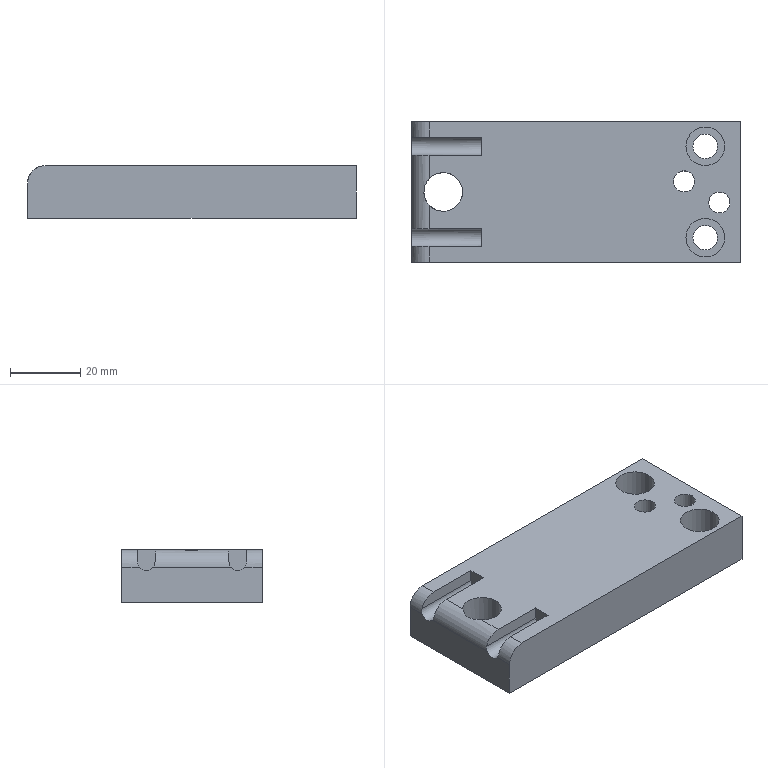Part | NX | features solid 2 | 1 solid | 26 faces | box 93.5 x 40 x 15 mm | volume 50400 mm3 | plane 14 | cylinder 12 | commonest cylinder face diameters 10 x3 11 x3 5 x2 6.001 x2 7 x2
STEP:
#1=CARTESIAN_POINT('',(481.,-15.5,-5.));
#2=VERTEX_POINT('',#1);
#3=CARTESIAN_POINT('',(481.,-10.5,-5.));
#4=VERTEX_POINT('',#3);
#5=CARTESIAN_POINT('',(481.,-13.,-5.));
#6=DIRECTION('',(1.,0.,0.));
#7=DIRECTION('',(0.,0.,1.));
#8=AXIS2_PLACEMENT_3D('',#5,#6,#7);
#9=CIRCLE('',#8,2.5);
#10=EDGE_CURVE('',#2,#4,#9,.T.);
#11=ORIENTED_EDGE('',*,*,#10,.F.);
#12=CARTESIAN_POINT('',(481.,-15.5,-1.5));
#13=VERTEX_POINT('',#12);
#14=CARTESIAN_POINT('',(481.,-15.5,25.));
#15=DIRECTION('',(0.,0.,-1.));
#16=VECTOR('',#15,1000.);
#17=LINE('',#14,#16);
#18=EDGE_CURVE('',#2,#13,#17,.F.);
#19=ORIENTED_EDGE('',*,*,#18,.T.);
#20=CARTESIAN_POINT('',(481.,-10.5,-1.5));
#21=VERTEX_POINT('',#20);
#22=CARTESIAN_POINT('',(481.,0.,-1.5));
#23=DIRECTION('',(0.,-1.,0.));
#24=VECTOR('',#23,1000.);
#25=LINE('',#22,#24);
#26=EDGE_CURVE('',#21,#13,#25,.T.);
#27=ORIENTED_EDGE('',*,*,#26,.F.);
#28=CARTESIAN_POINT('',(481.,-10.5,25.));
#29=DIRECTION('',(0.,0.,-1.));
#30=VECTOR('',#29,1000.);
#31=LINE('',#28,#30);
#32=EDGE_CURVE('',#4,#21,#31,.F.);
#33=ORIENTED_EDGE('',*,*,#32,.F.);
#34=EDGE_LOOP('',(#11,#19,#27,#33));
#35=FACE_BOUND('',#34,.T.);
#36=CARTESIAN_POINT('',(481.,-13.,-5.));
#37=DIRECTION('',(-1.,0.,0.));
#38=DIRECTION('',(0.,0.,1.));
#39=AXIS2_PLACEMENT_3D('',#36,#37,#38);
#40=PLANE('',#39);
#41=ADVANCED_FACE('',(#35),#40,.T.);
#42=CARTESIAN_POINT('',(461.,-11.,-6.5));
#43=VERTEX_POINT('',#42);
#44=CARTESIAN_POINT('',(461.23,-10.5,-5.));
#45=VERTEX_POINT('',#44);
#46=CARTESIAN_POINT('',(461.,-11.,-6.5));
#47=CARTESIAN_POINT('',(461.,-10.671,-6.061));
#48=CARTESIAN_POINT('',(461.066,-10.5,-5.521));
#49=CARTESIAN_POINT('',(461.23,-10.5,-5.));
#50=B_SPLINE_CURVE_WITH_KNOTS('',3,(#46,#47,#48,#49),.UNSPECIFIED.,.F.,.F.,(4,4),(0.,0.001624),.UNSPECIFIED.);
#51=EDGE_CURVE('',#43,#45,#50,.T.);
#52=ORIENTED_EDGE('',*,*,#51,.F.);
#53=CARTESIAN_POINT('',(461.,-15.,-6.5));
#54=VERTEX_POINT('',#53);
#55=CARTESIAN_POINT('',(461.,-13.,-5.));
#56=DIRECTION('',(-1.,0.,0.));
#57=DIRECTION('',(0.,0.,1.));
#58=AXIS2_PLACEMENT_3D('',#55,#56,#57);
#59=CIRCLE('',#58,2.5);
#60=EDGE_CURVE('',#54,#43,#59,.F.);
#61=ORIENTED_EDGE('',*,*,#60,.F.);
#62=CARTESIAN_POINT('',(461.23,-15.5,-5.));
#63=VERTEX_POINT('',#62);
#64=CARTESIAN_POINT('',(461.23,-15.5,-5.));
#65=CARTESIAN_POINT('',(461.068,-15.5,-5.516));
#66=CARTESIAN_POINT('',(461.,-15.329,-6.061));
#67=CARTESIAN_POINT('',(461.,-15.,-6.5));
#68=B_SPLINE_CURVE_WITH_KNOTS('',3,(#64,#65,#66,#67),.UNSPECIFIED.,.F.,.F.,(4,4),(0.01027,0.01189),.UNSPECIFIED.);
#69=EDGE_CURVE('',#63,#54,#68,.T.);
#70=ORIENTED_EDGE('',*,*,#69,.F.);
#71=CARTESIAN_POINT('',(451.,-15.5,-5.));
#72=DIRECTION('',(1.,0.,0.));
#73=VECTOR('',#72,1000.);
#74=LINE('',#71,#73);
#75=EDGE_CURVE('',#2,#63,#74,.F.);
#76=ORIENTED_EDGE('',*,*,#75,.F.);
#77=ORIENTED_EDGE('',*,*,#10,.T.);
#78=CARTESIAN_POINT('',(451.,-10.5,-5.));
#79=DIRECTION('',(1.,0.,0.));
#80=VECTOR('',#79,1000.);
#81=LINE('',#78,#80);
#82=EDGE_CURVE('',#45,#4,#81,.T.);
#83=ORIENTED_EDGE('',*,*,#82,.F.);
#84=EDGE_LOOP('',(#52,#61,#70,#76,#77,#83));
#85=FACE_BOUND('',#84,.T.);
#86=CARTESIAN_POINT('',(427.633,-13.,-5.));
#87=DIRECTION('',(1.,0.,0.));
#88=DIRECTION('',(0.,0.,-1.));
#89=AXIS2_PLACEMENT_3D('',#86,#87,#88);
#90=CYLINDRICAL_SURFACE('',#89,2.5);
#91=ADVANCED_FACE('',(#85),#90,.F.);
#92=CARTESIAN_POINT('',(466.,-10.5,-1.5));
#93=VERTEX_POINT('',#92);
#94=CARTESIAN_POINT('',(466.,-10.5,-6.5));
#95=DIRECTION('',(0.,1.,0.));
#96=DIRECTION('',(0.,0.,1.));
#97=AXIS2_PLACEMENT_3D('',#94,#95,#96);
#98=CIRCLE('',#97,5.);
#99=EDGE_CURVE('',#93,#45,#98,.F.);
#100=ORIENTED_EDGE('',*,*,#99,.T.);
#101=ORIENTED_EDGE('',*,*,#82,.T.);
#102=ORIENTED_EDGE('',*,*,#32,.T.);
#103=CARTESIAN_POINT('',(365.,-10.5,-1.5));
#104=DIRECTION('',(-1.,0.,0.));
#105=VECTOR('',#104,1000.);
#106=LINE('',#103,#105);
#107=EDGE_CURVE('',#21,#93,#106,.T.);
#108=ORIENTED_EDGE('',*,*,#107,.T.);
#109=EDGE_LOOP('',(#100,#101,#102,#108));
#110=FACE_BOUND('',#109,.T.);
#111=CARTESIAN_POINT('',(451.,-10.5,25.));
#112=DIRECTION('',(0.,1.,0.));
#113=DIRECTION('',(0.,0.,-1.));
#114=AXIS2_PLACEMENT_3D('',#111,#112,#113);
#115=PLANE('',#114);
#116=ADVANCED_FACE('',(#110),#115,.F.);
#117=CARTESIAN_POINT('',(466.,-15.5,-1.5));
#118=VERTEX_POINT('',#117);
#119=CARTESIAN_POINT('',(466.,-15.5,-6.5));
#120=DIRECTION('',(0.,-1.,0.));
#121=DIRECTION('',(0.,0.,-1.));
#122=AXIS2_PLACEMENT_3D('',#119,#120,#121);
#123=CIRCLE('',#122,5.);
#124=EDGE_CURVE('',#63,#118,#123,.F.);
#125=ORIENTED_EDGE('',*,*,#124,.T.);
#126=CARTESIAN_POINT('',(365.,-15.5,-1.5));
#127=DIRECTION('',(1.,0.,0.));
#128=VECTOR('',#127,1000.);
#129=LINE('',#126,#128);
#130=EDGE_CURVE('',#118,#13,#129,.T.);
#131=ORIENTED_EDGE('',*,*,#130,.T.);
#132=ORIENTED_EDGE('',*,*,#18,.F.);
#133=ORIENTED_EDGE('',*,*,#75,.T.);
#134=EDGE_LOOP('',(#125,#131,#132,#133));
#135=FACE_BOUND('',#134,.T.);
#136=CARTESIAN_POINT('',(451.,-15.5,25.));
#137=DIRECTION('',(0.,-1.,0.));
#138=DIRECTION('',(0.,0.,1.));
#139=AXIS2_PLACEMENT_3D('',#136,#137,#138);
#140=PLANE('',#139);
#141=ADVANCED_FACE('',(#135),#140,.F.);
#142=CARTESIAN_POINT('',(461.,11.,-6.5));
#143=VERTEX_POINT('',#142);
#144=CARTESIAN_POINT('',(461.,-29.,-6.5));
#145=DIRECTION('',(0.,-1.,0.));
#146=VECTOR('',#145,1000.);
#147=LINE('',#144,#146);
#148=EDGE_CURVE('',#43,#143,#147,.F.);
#149=ORIENTED_EDGE('',*,*,#148,.F.);
#150=ORIENTED_EDGE('',*,*,#51,.T.);
#151=ORIENTED_EDGE('',*,*,#99,.F.);
#152=CARTESIAN_POINT('',(466.,-3.775,-1.5));
#153=VERTEX_POINT('',#152);
#154=CARTESIAN_POINT('',(466.,0.,-1.5));
#155=DIRECTION('',(0.,-1.,0.));
#156=VECTOR('',#155,1000.);
#157=LINE('',#154,#156);
#158=EDGE_CURVE('',#153,#93,#157,.T.);
#159=ORIENTED_EDGE('',*,*,#158,.F.);
#160=CARTESIAN_POINT('',(466.,3.775,-1.5));
#161=VERTEX_POINT('',#160);
#162=CARTESIAN_POINT('',(466.,3.775,-1.5));
#163=CARTESIAN_POINT('',(465.037,2.755,-1.5));
#164=CARTESIAN_POINT('',(463.963,0.004291,-1.961));
#165=CARTESIAN_POINT('',(465.038,-2.755,-1.5));
#166=CARTESIAN_POINT('',(466.,-3.775,-1.5));
#167=B_SPLINE_CURVE_WITH_KNOTS('',3,(#162,#163,#164,#165,#166),.UNSPECIFIED.,.F.,.F.,(4,1,4),(0.,0.004144,0.008289),.UNSPECIFIED.);
#168=EDGE_CURVE('',#161,#153,#167,.T.);
#169=ORIENTED_EDGE('',*,*,#168,.F.);
#170=CARTESIAN_POINT('',(466.,10.5,-1.5));
#171=VERTEX_POINT('',#170);
#172=CARTESIAN_POINT('',(466.,0.,-1.5));
#173=DIRECTION('',(0.,-1.,0.));
#174=VECTOR('',#173,1000.);
#175=LINE('',#172,#174);
#176=EDGE_CURVE('',#171,#161,#175,.T.);
#177=ORIENTED_EDGE('',*,*,#176,.F.);
#178=CARTESIAN_POINT('',(461.23,10.5,-5.));
#179=VERTEX_POINT('',#178);
#180=CARTESIAN_POINT('',(466.,10.5,-6.5));
#181=DIRECTION('',(0.,-1.,0.));
#182=DIRECTION('',(0.,0.,-1.));
#183=AXIS2_PLACEMENT_3D('',#180,#181,#182);
#184=CIRCLE('',#183,5.);
#185=EDGE_CURVE('',#179,#171,#184,.F.);
#186=ORIENTED_EDGE('',*,*,#185,.F.);
#187=CARTESIAN_POINT('',(461.23,10.5,-5.));
#188=CARTESIAN_POINT('',(461.068,10.5,-5.516));
#189=CARTESIAN_POINT('',(461.,10.671,-6.061));
#190=CARTESIAN_POINT('',(461.,11.,-6.5));
#191=B_SPLINE_CURVE_WITH_KNOTS('',3,(#187,#188,#189,#190),.UNSPECIFIED.,.F.,.F.,(4,4),(0.01027,0.01189),.UNSPECIFIED.);
#192=EDGE_CURVE('',#179,#143,#191,.T.);
#193=ORIENTED_EDGE('',*,*,#192,.T.);
#194=EDGE_LOOP('',(#149,#150,#151,#159,#169,#177,#186,#193));
#195=FACE_BOUND('',#194,.T.);
#196=CARTESIAN_POINT('',(466.,0.,-6.5));
#197=DIRECTION('',(0.,-1.,0.));
#198=DIRECTION('',(0.,0.,-1.));
#199=AXIS2_PLACEMENT_3D('',#196,#197,#198);
#200=CYLINDRICAL_SURFACE('',#199,5.);
#201=ADVANCED_FACE('',(#195),#200,.T.);
#202=ORIENTED_EDGE('',*,*,#124,.F.);
#203=ORIENTED_EDGE('',*,*,#69,.T.);
#204=CARTESIAN_POINT('',(461.,-20.,-6.5));
#205=VERTEX_POINT('',#204);
#206=CARTESIAN_POINT('',(461.,-29.,-6.5));
#207=DIRECTION('',(0.,-1.,0.));
#208=VECTOR('',#207,1000.);
#209=LINE('',#206,#208);
#210=EDGE_CURVE('',#205,#54,#209,.F.);
#211=ORIENTED_EDGE('',*,*,#210,.F.);
#212=CARTESIAN_POINT('',(466.,-20.,-1.5));
#213=VERTEX_POINT('',#212);
#214=CARTESIAN_POINT('',(466.,-20.,-6.5));
#215=DIRECTION('',(0.,-1.,0.));
#216=DIRECTION('',(0.,0.,-1.));
#217=AXIS2_PLACEMENT_3D('',#214,#215,#216);
#218=CIRCLE('',#217,5.);
#219=EDGE_CURVE('',#213,#205,#218,.T.);
#220=ORIENTED_EDGE('',*,*,#219,.F.);
#221=CARTESIAN_POINT('',(466.,0.,-1.5));
#222=DIRECTION('',(0.,-1.,0.));
#223=VECTOR('',#222,1000.);
#224=LINE('',#221,#223);
#225=EDGE_CURVE('',#118,#213,#224,.T.);
#226=ORIENTED_EDGE('',*,*,#225,.F.);
#227=EDGE_LOOP('',(#202,#203,#211,#220,#226));
#228=FACE_BOUND('',#227,.T.);
#229=CARTESIAN_POINT('',(466.,0.,-6.5));
#230=DIRECTION('',(0.,-1.,0.));
#231=DIRECTION('',(0.,0.,-1.));
#232=AXIS2_PLACEMENT_3D('',#229,#230,#231);
#233=CYLINDRICAL_SURFACE('',#232,5.);
#234=ADVANCED_FACE('',(#228),#233,.T.);
#235=ORIENTED_EDGE('',*,*,#210,.T.);
#236=ORIENTED_EDGE('',*,*,#60,.T.);
#237=ORIENTED_EDGE('',*,*,#148,.T.);
#238=CARTESIAN_POINT('',(461.,15.,-6.5));
#239=VERTEX_POINT('',#238);
#240=CARTESIAN_POINT('',(461.,13.,-5.));
#241=DIRECTION('',(-1.,0.,0.));
#242=DIRECTION('',(0.,0.,1.));
#243=AXIS2_PLACEMENT_3D('',#240,#241,#242);
#244=CIRCLE('',#243,2.5);
#245=EDGE_CURVE('',#143,#239,#244,.F.);
#246=ORIENTED_EDGE('',*,*,#245,.T.);
#247=CARTESIAN_POINT('',(461.,20.,-6.5));
#248=VERTEX_POINT('',#247);
#249=CARTESIAN_POINT('',(461.,-29.,-6.5));
#250=DIRECTION('',(0.,-1.,0.));
#251=VECTOR('',#250,1000.);
#252=LINE('',#249,#251);
#253=EDGE_CURVE('',#239,#248,#252,.F.);
#254=ORIENTED_EDGE('',*,*,#253,.T.);
#255=CARTESIAN_POINT('',(461.,20.,-16.5));
#256=VERTEX_POINT('',#255);
#257=CARTESIAN_POINT('',(461.,20.,-51.5));
#258=DIRECTION('',(0.,0.,1.));
#259=VECTOR('',#258,1000.);
#260=LINE('',#257,#259);
#261=EDGE_CURVE('',#256,#248,#260,.T.);
#262=ORIENTED_EDGE('',*,*,#261,.F.);
#263=CARTESIAN_POINT('',(461.,-20.,-16.5));
#264=VERTEX_POINT('',#263);
#265=CARTESIAN_POINT('',(461.,0.,-16.5));
#266=DIRECTION('',(0.,1.,0.));
#267=VECTOR('',#266,1000.);
#268=LINE('',#265,#267);
#269=EDGE_CURVE('',#264,#256,#268,.T.);
#270=ORIENTED_EDGE('',*,*,#269,.F.);
#271=CARTESIAN_POINT('',(461.,-20.,-51.5));
#272=DIRECTION('',(0.,0.,-1.));
#273=VECTOR('',#272,1000.);
#274=LINE('',#271,#273);
#275=EDGE_CURVE('',#205,#264,#274,.T.);
#276=ORIENTED_EDGE('',*,*,#275,.F.);
#277=EDGE_LOOP('',(#235,#236,#237,#246,#254,#262,#270,#276));
#278=FACE_BOUND('',#277,.T.);
#279=CARTESIAN_POINT('',(461.,-29.,0.));
#280=DIRECTION('',(-1.,0.,0.));
#281=DIRECTION('',(0.,0.,1.));
#282=AXIS2_PLACEMENT_3D('',#279,#280,#281);
#283=PLANE('',#282);
#284=ADVANCED_FACE('',(#278),#283,.T.);
#285=ORIENTED_EDGE('',*,*,#192,.F.);
#286=CARTESIAN_POINT('',(481.,10.5,-5.));
#287=VERTEX_POINT('',#286);
#288=CARTESIAN_POINT('',(451.,10.5,-5.));
#289=DIRECTION('',(1.,0.,0.));
#290=VECTOR('',#289,1000.);
#291=LINE('',#288,#290);
#292=EDGE_CURVE('',#287,#179,#291,.F.);
#293=ORIENTED_EDGE('',*,*,#292,.F.);
#294=CARTESIAN_POINT('',(481.,15.5,-5.));
#295=VERTEX_POINT('',#294);
#296=CARTESIAN_POINT('',(481.,13.,-5.));
#297=DIRECTION('',(-1.,0.,0.));
#298=DIRECTION('',(0.,0.,1.));
#299=AXIS2_PLACEMENT_3D('',#296,#297,#298);
#300=CIRCLE('',#299,2.5);
#301=EDGE_CURVE('',#287,#295,#300,.F.);
#302=ORIENTED_EDGE('',*,*,#301,.T.);
#303=CARTESIAN_POINT('',(461.23,15.5,-5.));
#304=VERTEX_POINT('',#303);
#305=CARTESIAN_POINT('',(451.,15.5,-5.));
#306=DIRECTION('',(1.,0.,0.));
#307=VECTOR('',#306,1000.);
#308=LINE('',#305,#307);
#309=EDGE_CURVE('',#304,#295,#308,.T.);
#310=ORIENTED_EDGE('',*,*,#309,.F.);
#311=CARTESIAN_POINT('',(461.,15.,-6.5));
#312=CARTESIAN_POINT('',(461.,15.329,-6.061));
#313=CARTESIAN_POINT('',(461.066,15.5,-5.521));
#314=CARTESIAN_POINT('',(461.23,15.5,-5.));
#315=B_SPLINE_CURVE_WITH_KNOTS('',3,(#311,#312,#313,#314),.UNSPECIFIED.,.F.,.F.,(4,4),(0.,0.001624),.UNSPECIFIED.);
#316=EDGE_CURVE('',#239,#304,#315,.T.);
#317=ORIENTED_EDGE('',*,*,#316,.F.);
#318=ORIENTED_EDGE('',*,*,#245,.F.);
#319=EDGE_LOOP('',(#285,#293,#302,#310,#317,#318));
#320=FACE_BOUND('',#319,.T.);
#321=CARTESIAN_POINT('',(427.633,13.,-5.));
#322=DIRECTION('',(1.,0.,0.));
#323=DIRECTION('',(0.,0.,-1.));
#324=AXIS2_PLACEMENT_3D('',#321,#322,#323);
#325=CYLINDRICAL_SURFACE('',#324,2.5);
#326=ADVANCED_FACE('',(#320),#325,.F.);
#327=CARTESIAN_POINT('',(466.,15.5,-1.5));
#328=VERTEX_POINT('',#327);
#329=CARTESIAN_POINT('',(466.,15.5,-6.5));
#330=DIRECTION('',(0.,1.,0.));
#331=DIRECTION('',(0.,0.,1.));
#332=AXIS2_PLACEMENT_3D('',#329,#330,#331);
#333=CIRCLE('',#332,5.);
#334=EDGE_CURVE('',#328,#304,#333,.F.);
#335=ORIENTED_EDGE('',*,*,#334,.F.);
#336=CARTESIAN_POINT('',(466.,20.,-1.5));
#337=VERTEX_POINT('',#336);
#338=CARTESIAN_POINT('',(466.,0.,-1.5));
#339=DIRECTION('',(0.,-1.,0.));
#340=VECTOR('',#339,1000.);
#341=LINE('',#338,#340);
#342=EDGE_CURVE('',#337,#328,#341,.T.);
#343=ORIENTED_EDGE('',*,*,#342,.F.);
#344=CARTESIAN_POINT('',(466.,20.,-6.5));
#345=DIRECTION('',(0.,1.,0.));
#346=DIRECTION('',(0.,0.,1.));
#347=AXIS2_PLACEMENT_3D('',#344,#345,#346);
#348=CIRCLE('',#347,5.);
#349=EDGE_CURVE('',#248,#337,#348,.T.);
#350=ORIENTED_EDGE('',*,*,#349,.F.);
#351=ORIENTED_EDGE('',*,*,#253,.F.);
#352=ORIENTED_EDGE('',*,*,#316,.T.);
#353=EDGE_LOOP('',(#335,#343,#350,#351,#352));
#354=FACE_BOUND('',#353,.T.);
#355=CARTESIAN_POINT('',(466.,0.,-6.5));
#356=DIRECTION('',(0.,-1.,0.));
#357=DIRECTION('',(0.,0.,-1.));
#358=AXIS2_PLACEMENT_3D('',#355,#356,#357);
#359=CYLINDRICAL_SURFACE('',#358,5.);
#360=ADVANCED_FACE('',(#354),#359,.T.);
#361=ORIENTED_EDGE('',*,*,#107,.F.);
#362=ORIENTED_EDGE('',*,*,#26,.T.);
#363=ORIENTED_EDGE('',*,*,#130,.F.);
#364=ORIENTED_EDGE('',*,*,#225,.T.);
#365=CARTESIAN_POINT('',(554.5,-20.,-1.5));
#366=VERTEX_POINT('',#365);
#367=CARTESIAN_POINT('',(365.,-20.,-1.5));
#368=DIRECTION('',(-1.,0.,0.));
#369=VECTOR('',#368,1000.);
#370=LINE('',#367,#369);
#371=EDGE_CURVE('',#366,#213,#370,.T.);
#372=ORIENTED_EDGE('',*,*,#371,.F.);
#373=CARTESIAN_POINT('',(554.5,20.,-1.5));
#374=VERTEX_POINT('',#373);
#375=CARTESIAN_POINT('',(554.5,0.,-1.5));
#376=DIRECTION('',(0.,-1.,0.));
#377=VECTOR('',#376,1000.);
#378=LINE('',#375,#377);
#379=EDGE_CURVE('',#374,#366,#378,.T.);
#380=ORIENTED_EDGE('',*,*,#379,.F.);
#381=CARTESIAN_POINT('',(365.,20.,-1.5));
#382=DIRECTION('',(1.,0.,0.));
#383=VECTOR('',#382,1000.);
#384=LINE('',#381,#383);
#385=EDGE_CURVE('',#337,#374,#384,.T.);
#386=ORIENTED_EDGE('',*,*,#385,.F.);
#387=ORIENTED_EDGE('',*,*,#342,.T.);
#388=CARTESIAN_POINT('',(481.,15.5,-1.5));
#389=VERTEX_POINT('',#388);
#390=CARTESIAN_POINT('',(365.,15.5,-1.5));
#391=DIRECTION('',(-1.,0.,0.));
#392=VECTOR('',#391,1000.);
#393=LINE('',#390,#392);
#394=EDGE_CURVE('',#389,#328,#393,.T.);
#395=ORIENTED_EDGE('',*,*,#394,.F.);
#396=CARTESIAN_POINT('',(481.,10.5,-1.5));
#397=VERTEX_POINT('',#396);
#398=CARTESIAN_POINT('',(481.,0.,-1.5));
#399=DIRECTION('',(0.,-1.,0.));
#400=VECTOR('',#399,1000.);
#401=LINE('',#398,#400);
#402=EDGE_CURVE('',#389,#397,#401,.T.);
#403=ORIENTED_EDGE('',*,*,#402,.T.);
#404=CARTESIAN_POINT('',(365.,10.5,-1.5));
#405=DIRECTION('',(1.,0.,0.));
#406=VECTOR('',#405,1000.);
#407=LINE('',#404,#406);
#408=EDGE_CURVE('',#171,#397,#407,.T.);
#409=ORIENTED_EDGE('',*,*,#408,.F.);
#410=ORIENTED_EDGE('',*,*,#176,.T.);
#411=CARTESIAN_POINT('',(470.,0.,-1.5));
#412=DIRECTION('',(0.,0.,1.));
#413=DIRECTION('',(1.,0.,0.));
#414=AXIS2_PLACEMENT_3D('',#411,#412,#413);
#415=CIRCLE('',#414,5.5);
#416=EDGE_CURVE('',#153,#161,#415,.T.);
#417=ORIENTED_EDGE('',*,*,#416,.F.);
#418=ORIENTED_EDGE('',*,*,#158,.T.);
#419=EDGE_LOOP('',(#361,#362,#363,#364,#372,#380,#386,#387,#395,#403,#409,#410,#417,#418));
#420=FACE_BOUND('',#419,.T.);
#421=CARTESIAN_POINT('',(551.5,-3.,-1.5));
#422=VERTEX_POINT('',#421);
#423=CARTESIAN_POINT('',(548.5,-3.,-1.5));
#424=DIRECTION('',(0.,0.,1.));
#425=DIRECTION('',(1.,0.,0.));
#426=AXIS2_PLACEMENT_3D('',#423,#424,#425);
#427=CIRCLE('',#426,3.001);
#428=EDGE_CURVE('',#422,#422,#427,.T.);
#429=ORIENTED_EDGE('',*,*,#428,.F.);
#430=EDGE_LOOP('',(#429));
#431=FACE_BOUND('',#430,.T.);
#432=CARTESIAN_POINT('',(541.5,3.,-1.5));
#433=VERTEX_POINT('',#432);
#434=CARTESIAN_POINT('',(538.5,3.,-1.5));
#435=DIRECTION('',(0.,0.,1.));
#436=DIRECTION('',(1.,0.,0.));
#437=AXIS2_PLACEMENT_3D('',#434,#435,#436);
#438=CIRCLE('',#437,3.001);
#439=EDGE_CURVE('',#433,#433,#438,.T.);
#440=ORIENTED_EDGE('',*,*,#439,.F.);
#441=EDGE_LOOP('',(#440));
#442=FACE_BOUND('',#441,.T.);
#443=CARTESIAN_POINT('',(550.,-13.,-1.5));
#444=VERTEX_POINT('',#443);
#445=CARTESIAN_POINT('',(544.5,-13.,-1.5));
#446=DIRECTION('',(0.,0.,1.));
#447=DIRECTION('',(1.,0.,0.));
#448=AXIS2_PLACEMENT_3D('',#445,#446,#447);
#449=CIRCLE('',#448,5.5);
#450=EDGE_CURVE('',#444,#444,#449,.T.);
#451=ORIENTED_EDGE('',*,*,#450,.F.);
#452=EDGE_LOOP('',(#451));
#453=FACE_BOUND('',#452,.T.);
#454=CARTESIAN_POINT('',(550.,13.,-1.5));
#455=VERTEX_POINT('',#454);
#456=CARTESIAN_POINT('',(544.5,13.,-1.5));
#457=DIRECTION('',(0.,0.,-1.));
#458=DIRECTION('',(1.,0.,0.));
#459=AXIS2_PLACEMENT_3D('',#456,#457,#458);
#460=CIRCLE('',#459,5.5);
#461=EDGE_CURVE('',#455,#455,#460,.T.);
#462=ORIENTED_EDGE('',*,*,#461,.T.);
#463=EDGE_LOOP('',(#462));
#464=FACE_BOUND('',#463,.T.);
#465=CARTESIAN_POINT('',(365.,0.,-1.5));
#466=DIRECTION('',(0.,0.,1.));
#467=DIRECTION('',(1.,0.,0.));
#468=AXIS2_PLACEMENT_3D('',#465,#466,#467);
#469=PLANE('',#468);
#470=ADVANCED_FACE('',(#420,#431,#442,#453,#464),#469,.T.);
#471=ORIENTED_EDGE('',*,*,#261,.T.);
#472=ORIENTED_EDGE('',*,*,#349,.T.);
#473=ORIENTED_EDGE('',*,*,#385,.T.);
#474=CARTESIAN_POINT('',(554.5,20.,-16.5));
#475=VERTEX_POINT('',#474);
#476=CARTESIAN_POINT('',(554.5,20.,-51.5));
#477=DIRECTION('',(0.,0.,1.));
#478=VECTOR('',#477,1000.);
#479=LINE('',#476,#478);
#480=EDGE_CURVE('',#475,#374,#479,.T.);
#481=ORIENTED_EDGE('',*,*,#480,.F.);
#482=CARTESIAN_POINT('',(365.,20.,-16.5));
#483=DIRECTION('',(-1.,0.,0.));
#484=VECTOR('',#483,1000.);
#485=LINE('',#482,#484);
#486=EDGE_CURVE('',#475,#256,#485,.T.);
#487=ORIENTED_EDGE('',*,*,#486,.T.);
#488=EDGE_LOOP('',(#471,#472,#473,#481,#487));
#489=FACE_BOUND('',#488,.T.);
#490=CARTESIAN_POINT('',(365.,20.,-51.5));
#491=DIRECTION('',(0.,1.,0.));
#492=DIRECTION('',(0.,0.,1.));
#493=AXIS2_PLACEMENT_3D('',#490,#491,#492);
#494=PLANE('',#493);
#495=ADVANCED_FACE('',(#489),#494,.T.);
#496=ORIENTED_EDGE('',*,*,#371,.T.);
#497=ORIENTED_EDGE('',*,*,#219,.T.);
#498=ORIENTED_EDGE('',*,*,#275,.T.);
#499=CARTESIAN_POINT('',(554.5,-20.,-16.5));
#500=VERTEX_POINT('',#499);
#501=CARTESIAN_POINT('',(365.,-20.,-16.5));
#502=DIRECTION('',(1.,0.,0.));
#503=VECTOR('',#502,1000.);
#504=LINE('',#501,#503);
#505=EDGE_CURVE('',#264,#500,#504,.T.);
#506=ORIENTED_EDGE('',*,*,#505,.T.);
#507=CARTESIAN_POINT('',(554.5,-20.,-51.5));
#508=DIRECTION('',(0.,0.,1.));
#509=VECTOR('',#508,1000.);
#510=LINE('',#507,#509);
#511=EDGE_CURVE('',#500,#366,#510,.T.);
#512=ORIENTED_EDGE('',*,*,#511,.T.);
#513=EDGE_LOOP('',(#496,#497,#498,#506,#512));
#514=FACE_BOUND('',#513,.T.);
#515=CARTESIAN_POINT('',(365.,-20.,-51.5));
#516=DIRECTION('',(0.,-1.,0.));
#517=DIRECTION('',(0.,0.,-1.));
#518=AXIS2_PLACEMENT_3D('',#515,#516,#517);
#519=PLANE('',#518);
#520=ADVANCED_FACE('',(#514),#519,.T.);
#521=CARTESIAN_POINT('',(464.5,0.,-16.5));
#522=VERTEX_POINT('',#521);
#523=CARTESIAN_POINT('',(470.,0.,-16.5));
#524=DIRECTION('',(0.,0.,-1.));
#525=DIRECTION('',(-1.,0.,0.));
#526=AXIS2_PLACEMENT_3D('',#523,#524,#525);
#527=CIRCLE('',#526,5.5);
#528=EDGE_CURVE('',#522,#522,#527,.T.);
#529=ORIENTED_EDGE('',*,*,#528,.F.);
#530=EDGE_LOOP('',(#529));
#531=FACE_BOUND('',#530,.T.);
#532=CARTESIAN_POINT('',(545.5,-3.,-16.5));
#533=VERTEX_POINT('',#532);
#534=CARTESIAN_POINT('',(548.5,-3.,-16.5));
#535=DIRECTION('',(0.,0.,-1.));
#536=DIRECTION('',(-1.,0.,0.));
#537=AXIS2_PLACEMENT_3D('',#534,#535,#536);
#538=CIRCLE('',#537,3.001);
#539=EDGE_CURVE('',#533,#533,#538,.T.);
#540=ORIENTED_EDGE('',*,*,#539,.F.);
#541=EDGE_LOOP('',(#540));
#542=FACE_BOUND('',#541,.T.);
#543=CARTESIAN_POINT('',(535.5,3.,-16.5));
#544=VERTEX_POINT('',#543);
#545=CARTESIAN_POINT('',(538.5,3.,-16.5));
#546=DIRECTION('',(0.,0.,-1.));
#547=DIRECTION('',(-1.,0.,0.));
#548=AXIS2_PLACEMENT_3D('',#545,#546,#547);
#549=CIRCLE('',#548,3.001);
#550=EDGE_CURVE('',#544,#544,#549,.T.);
#551=ORIENTED_EDGE('',*,*,#550,.F.);
#552=EDGE_LOOP('',(#551));
#553=FACE_BOUND('',#552,.T.);
#554=CARTESIAN_POINT('',(541.,-13.,-16.5));
#555=VERTEX_POINT('',#554);
#556=CARTESIAN_POINT('',(544.5,-13.,-16.5));
#557=DIRECTION('',(0.,0.,-1.));
#558=DIRECTION('',(-1.,0.,0.));
#559=AXIS2_PLACEMENT_3D('',#556,#557,#558);
#560=CIRCLE('',#559,3.5);
#561=EDGE_CURVE('',#555,#555,#560,.T.);
#562=ORIENTED_EDGE('',*,*,#561,.F.);
#563=EDGE_LOOP('',(#562));
#564=FACE_BOUND('',#563,.T.);
#565=CARTESIAN_POINT('',(541.,13.,-16.5));
#566=VERTEX_POINT('',#565);
#567=CARTESIAN_POINT('',(544.5,13.,-16.5));
#568=DIRECTION('',(0.,0.,-1.));
#569=DIRECTION('',(-1.,0.,0.));
#570=AXIS2_PLACEMENT_3D('',#567,#568,#569);
#571=CIRCLE('',#570,3.5);
#572=EDGE_CURVE('',#566,#566,#571,.T.);
#573=ORIENTED_EDGE('',*,*,#572,.F.);
#574=EDGE_LOOP('',(#573));
#575=FACE_BOUND('',#574,.T.);
#576=ORIENTED_EDGE('',*,*,#505,.F.);
#577=ORIENTED_EDGE('',*,*,#269,.T.);
#578=ORIENTED_EDGE('',*,*,#486,.F.);
#579=CARTESIAN_POINT('',(554.5,0.,-16.5));
#580=DIRECTION('',(0.,1.,0.));
#581=VECTOR('',#580,1000.);
#582=LINE('',#579,#581);
#583=EDGE_CURVE('',#500,#475,#582,.T.);
#584=ORIENTED_EDGE('',*,*,#583,.F.);
#585=EDGE_LOOP('',(#576,#577,#578,#584));
#586=FACE_BOUND('',#585,.T.);
#587=CARTESIAN_POINT('',(386.,0.,-16.5));
#588=DIRECTION('',(0.,0.,-1.));
#589=DIRECTION('',(-1.,0.,0.));
#590=AXIS2_PLACEMENT_3D('',#587,#588,#589);
#591=PLANE('',#590);
#592=ADVANCED_FACE('',(#531,#542,#553,#564,#575,#586),#591,.T.);
#593=ORIENTED_EDGE('',*,*,#511,.F.);
#594=ORIENTED_EDGE('',*,*,#583,.T.);
#595=ORIENTED_EDGE('',*,*,#480,.T.);
#596=ORIENTED_EDGE('',*,*,#379,.T.);
#597=EDGE_LOOP('',(#593,#594,#595,#596));
#598=FACE_BOUND('',#597,.T.);
#599=CARTESIAN_POINT('',(554.5,0.,-51.5));
#600=DIRECTION('',(1.,0.,0.));
#601=DIRECTION('',(0.,0.,-1.));
#602=AXIS2_PLACEMENT_3D('',#599,#600,#601);
#603=PLANE('',#602);
#604=ADVANCED_FACE('',(#598),#603,.T.);
#605=ORIENTED_EDGE('',*,*,#572,.T.);
#606=EDGE_LOOP('',(#605));
#607=FACE_BOUND('',#606,.T.);
#608=CARTESIAN_POINT('',(541.,13.,-10.5));
#609=VERTEX_POINT('',#608);
#610=CARTESIAN_POINT('',(544.5,13.,-10.5));
#611=DIRECTION('',(0.,0.,-1.));
#612=DIRECTION('',(-1.,0.,0.));
#613=AXIS2_PLACEMENT_3D('',#610,#611,#612);
#614=CIRCLE('',#613,3.5);
#615=EDGE_CURVE('',#609,#609,#614,.T.);
#616=ORIENTED_EDGE('',*,*,#615,.F.);
#617=EDGE_LOOP('',(#616));
#618=FACE_BOUND('',#617,.T.);
#619=CARTESIAN_POINT('',(544.5,13.,0.5));
#620=DIRECTION('',(0.,0.,-1.));
#621=DIRECTION('',(1.,0.,0.));
#622=AXIS2_PLACEMENT_3D('',#619,#620,#621);
#623=CYLINDRICAL_SURFACE('',#622,3.5);
#624=ADVANCED_FACE('',(#607,#618),#623,.F.);
#625=ORIENTED_EDGE('',*,*,#615,.T.);
#626=EDGE_LOOP('',(#625));
#627=FACE_BOUND('',#626,.T.);
#628=CARTESIAN_POINT('',(550.,13.,-10.5));
#629=VERTEX_POINT('',#628);
#630=CARTESIAN_POINT('',(544.5,13.,-10.5));
#631=DIRECTION('',(0.,0.,1.));
#632=DIRECTION('',(1.,0.,0.));
#633=AXIS2_PLACEMENT_3D('',#630,#631,#632);
#634=CIRCLE('',#633,5.5);
#635=EDGE_CURVE('',#629,#629,#634,.F.);
#636=ORIENTED_EDGE('',*,*,#635,.F.);
#637=EDGE_LOOP('',(#636));
#638=FACE_BOUND('',#637,.T.);
#639=CARTESIAN_POINT('',(544.5,13.,-10.5));
#640=DIRECTION('',(0.,0.,-1.));
#641=DIRECTION('',(-1.,0.,0.));
#642=AXIS2_PLACEMENT_3D('',#639,#640,#641);
#643=PLANE('',#642);
#644=ADVANCED_FACE('',(#627,#638),#643,.F.);
#645=ORIENTED_EDGE('',*,*,#635,.T.);
#646=EDGE_LOOP('',(#645));
#647=FACE_BOUND('',#646,.T.);
#648=ORIENTED_EDGE('',*,*,#461,.F.);
#649=EDGE_LOOP('',(#648));
#650=FACE_BOUND('',#649,.T.);
#651=CARTESIAN_POINT('',(544.5,13.,-1.5));
#652=DIRECTION('',(0.,0.,-1.));
#653=DIRECTION('',(1.,0.,0.));
#654=AXIS2_PLACEMENT_3D('',#651,#652,#653);
#655=CYLINDRICAL_SURFACE('',#654,5.5);
#656=ADVANCED_FACE('',(#647,#650),#655,.F.);
#657=ORIENTED_EDGE('',*,*,#561,.T.);
#658=EDGE_LOOP('',(#657));
#659=FACE_BOUND('',#658,.T.);
#660=CARTESIAN_POINT('',(541.,-13.,-10.5));
#661=VERTEX_POINT('',#660);
#662=CARTESIAN_POINT('',(544.5,-13.,-10.5));
#663=DIRECTION('',(0.,0.,1.));
#664=DIRECTION('',(-1.,0.,0.));
#665=AXIS2_PLACEMENT_3D('',#662,#663,#664);
#666=CIRCLE('',#665,3.5);
#667=EDGE_CURVE('',#661,#661,#666,.T.);
#668=ORIENTED_EDGE('',*,*,#667,.T.);
#669=EDGE_LOOP('',(#668));
#670=FACE_BOUND('',#669,.T.);
#671=CARTESIAN_POINT('',(544.5,-13.,0.5));
#672=DIRECTION('',(0.,0.,-1.));
#673=DIRECTION('',(1.,0.,0.));
#674=AXIS2_PLACEMENT_3D('',#671,#672,#673);
#675=CYLINDRICAL_SURFACE('',#674,3.5);
#676=ADVANCED_FACE('',(#659,#670),#675,.F.);
#677=ORIENTED_EDGE('',*,*,#667,.F.);
#678=EDGE_LOOP('',(#677));
#679=FACE_BOUND('',#678,.T.);
#680=CARTESIAN_POINT('',(550.,-13.,-10.5));
#681=VERTEX_POINT('',#680);
#682=CARTESIAN_POINT('',(544.5,-13.,-10.5));
#683=DIRECTION('',(0.,0.,-1.));
#684=DIRECTION('',(1.,0.,0.));
#685=AXIS2_PLACEMENT_3D('',#682,#683,#684);
#686=CIRCLE('',#685,5.5);
#687=EDGE_CURVE('',#681,#681,#686,.F.);
#688=ORIENTED_EDGE('',*,*,#687,.T.);
#689=EDGE_LOOP('',(#688));
#690=FACE_BOUND('',#689,.T.);
#691=CARTESIAN_POINT('',(544.5,-13.,-10.5));
#692=DIRECTION('',(0.,0.,-1.));
#693=DIRECTION('',(-1.,0.,0.));
#694=AXIS2_PLACEMENT_3D('',#691,#692,#693);
#695=PLANE('',#694);
#696=ADVANCED_FACE('',(#679,#690),#695,.F.);
#697=ORIENTED_EDGE('',*,*,#687,.F.);
#698=EDGE_LOOP('',(#697));
#699=FACE_BOUND('',#698,.T.);
#700=ORIENTED_EDGE('',*,*,#450,.T.);
#701=EDGE_LOOP('',(#700));
#702=FACE_BOUND('',#701,.T.);
#703=CARTESIAN_POINT('',(544.5,-13.,-1.5));
#704=DIRECTION('',(0.,0.,-1.));
#705=DIRECTION('',(1.,0.,0.));
#706=AXIS2_PLACEMENT_3D('',#703,#704,#705);
#707=CYLINDRICAL_SURFACE('',#706,5.5);
#708=ADVANCED_FACE('',(#699,#702),#707,.F.);
#709=ORIENTED_EDGE('',*,*,#439,.T.);
#710=EDGE_LOOP('',(#709));
#711=FACE_BOUND('',#710,.T.);
#712=ORIENTED_EDGE('',*,*,#550,.T.);
#713=EDGE_LOOP('',(#712));
#714=FACE_BOUND('',#713,.T.);
#715=CARTESIAN_POINT('',(538.5,3.,0.5));
#716=DIRECTION('',(0.,0.,-1.));
#717=DIRECTION('',(-1.,0.,0.));
#718=AXIS2_PLACEMENT_3D('',#715,#716,#717);
#719=CYLINDRICAL_SURFACE('',#718,3.001);
#720=ADVANCED_FACE('',(#711,#714),#719,.F.);
#721=ORIENTED_EDGE('',*,*,#428,.T.);
#722=EDGE_LOOP('',(#721));
#723=FACE_BOUND('',#722,.T.);
#724=ORIENTED_EDGE('',*,*,#539,.T.);
#725=EDGE_LOOP('',(#724));
#726=FACE_BOUND('',#725,.T.);
#727=CARTESIAN_POINT('',(548.5,-3.,0.5));
#728=DIRECTION('',(0.,0.,-1.));
#729=DIRECTION('',(1.,0.,0.));
#730=AXIS2_PLACEMENT_3D('',#727,#728,#729);
#731=CYLINDRICAL_SURFACE('',#730,3.001);
#732=ADVANCED_FACE('',(#723,#726),#731,.F.);
#733=ORIENTED_EDGE('',*,*,#416,.T.);
#734=ORIENTED_EDGE('',*,*,#168,.T.);
#735=EDGE_LOOP('',(#733,#734));
#736=FACE_BOUND('',#735,.T.);
#737=ORIENTED_EDGE('',*,*,#528,.T.);
#738=EDGE_LOOP('',(#737));
#739=FACE_BOUND('',#738,.T.);
#740=CARTESIAN_POINT('',(470.,0.,-34.5));
#741=DIRECTION('',(0.,0.,1.));
#742=DIRECTION('',(1.,0.,0.));
#743=AXIS2_PLACEMENT_3D('',#740,#741,#742);
#744=CYLINDRICAL_SURFACE('',#743,5.5);
#745=ADVANCED_FACE('',(#736,#739),#744,.F.);
#746=ORIENTED_EDGE('',*,*,#301,.F.);
#747=CARTESIAN_POINT('',(481.,10.5,25.));
#748=DIRECTION('',(0.,0.,-1.));
#749=VECTOR('',#748,1000.);
#750=LINE('',#747,#749);
#751=EDGE_CURVE('',#397,#287,#750,.T.);
#752=ORIENTED_EDGE('',*,*,#751,.F.);
#753=ORIENTED_EDGE('',*,*,#402,.F.);
#754=CARTESIAN_POINT('',(481.,15.5,25.));
#755=DIRECTION('',(0.,0.,-1.));
#756=VECTOR('',#755,1000.);
#757=LINE('',#754,#756);
#758=EDGE_CURVE('',#389,#295,#757,.T.);
#759=ORIENTED_EDGE('',*,*,#758,.T.);
#760=EDGE_LOOP('',(#746,#752,#753,#759));
#761=FACE_BOUND('',#760,.T.);
#762=CARTESIAN_POINT('',(481.,13.,-5.));
#763=DIRECTION('',(-1.,0.,0.));
#764=DIRECTION('',(0.,0.,1.));
#765=AXIS2_PLACEMENT_3D('',#762,#763,#764);
#766=PLANE('',#765);
#767=ADVANCED_FACE('',(#761),#766,.T.);
#768=ORIENTED_EDGE('',*,*,#185,.T.);
#769=ORIENTED_EDGE('',*,*,#408,.T.);
#770=ORIENTED_EDGE('',*,*,#751,.T.);
#771=ORIENTED_EDGE('',*,*,#292,.T.);
#772=EDGE_LOOP('',(#768,#769,#770,#771));
#773=FACE_BOUND('',#772,.T.);
#774=CARTESIAN_POINT('',(451.,10.5,25.));
#775=DIRECTION('',(0.,-1.,0.));
#776=DIRECTION('',(0.,0.,-1.));
#777=AXIS2_PLACEMENT_3D('',#774,#775,#776);
#778=PLANE('',#777);
#779=ADVANCED_FACE('',(#773),#778,.F.);
#780=ORIENTED_EDGE('',*,*,#334,.T.);
#781=ORIENTED_EDGE('',*,*,#309,.T.);
#782=ORIENTED_EDGE('',*,*,#758,.F.);
#783=ORIENTED_EDGE('',*,*,#394,.T.);
#784=EDGE_LOOP('',(#780,#781,#782,#783));
#785=FACE_BOUND('',#784,.T.);
#786=CARTESIAN_POINT('',(451.,15.5,25.));
#787=DIRECTION('',(0.,1.,0.));
#788=DIRECTION('',(0.,0.,1.));
#789=AXIS2_PLACEMENT_3D('',#786,#787,#788);
#790=PLANE('',#789);
#791=ADVANCED_FACE('',(#785),#790,.F.);
#792=CLOSED_SHELL('',(#41,#91,#116,#141,#201,#234,#284,#326,#360,#470,#495,#520,#592,#604,#624,#644,#656,#676,#696,#708,#720,#732,#745,#767,#779,#791));
#793=MANIFOLD_SOLID_BREP('',#792);
#794=(LENGTH_UNIT()NAMED_UNIT(*)SI_UNIT(.MILLI.,.METRE.));
#795=UNCERTAINTY_MEASURE_WITH_UNIT(LENGTH_MEASURE(0.0508),#794,'','');
#796=(NAMED_UNIT(*)PLANE_ANGLE_UNIT()SI_UNIT($,.RADIAN.));
#797=(NAMED_UNIT(*)SI_UNIT($,.STERADIAN.)SOLID_ANGLE_UNIT());
#798=(GEOMETRIC_REPRESENTATION_CONTEXT(3)GLOBAL_UNCERTAINTY_ASSIGNED_CONTEXT((#795))GLOBAL_UNIT_ASSIGNED_CONTEXT((#794,#796,#797))REPRESENTATION_CONTEXT('',''));
#799=ADVANCED_BREP_SHAPE_REPRESENTATION('',(#793),#798);